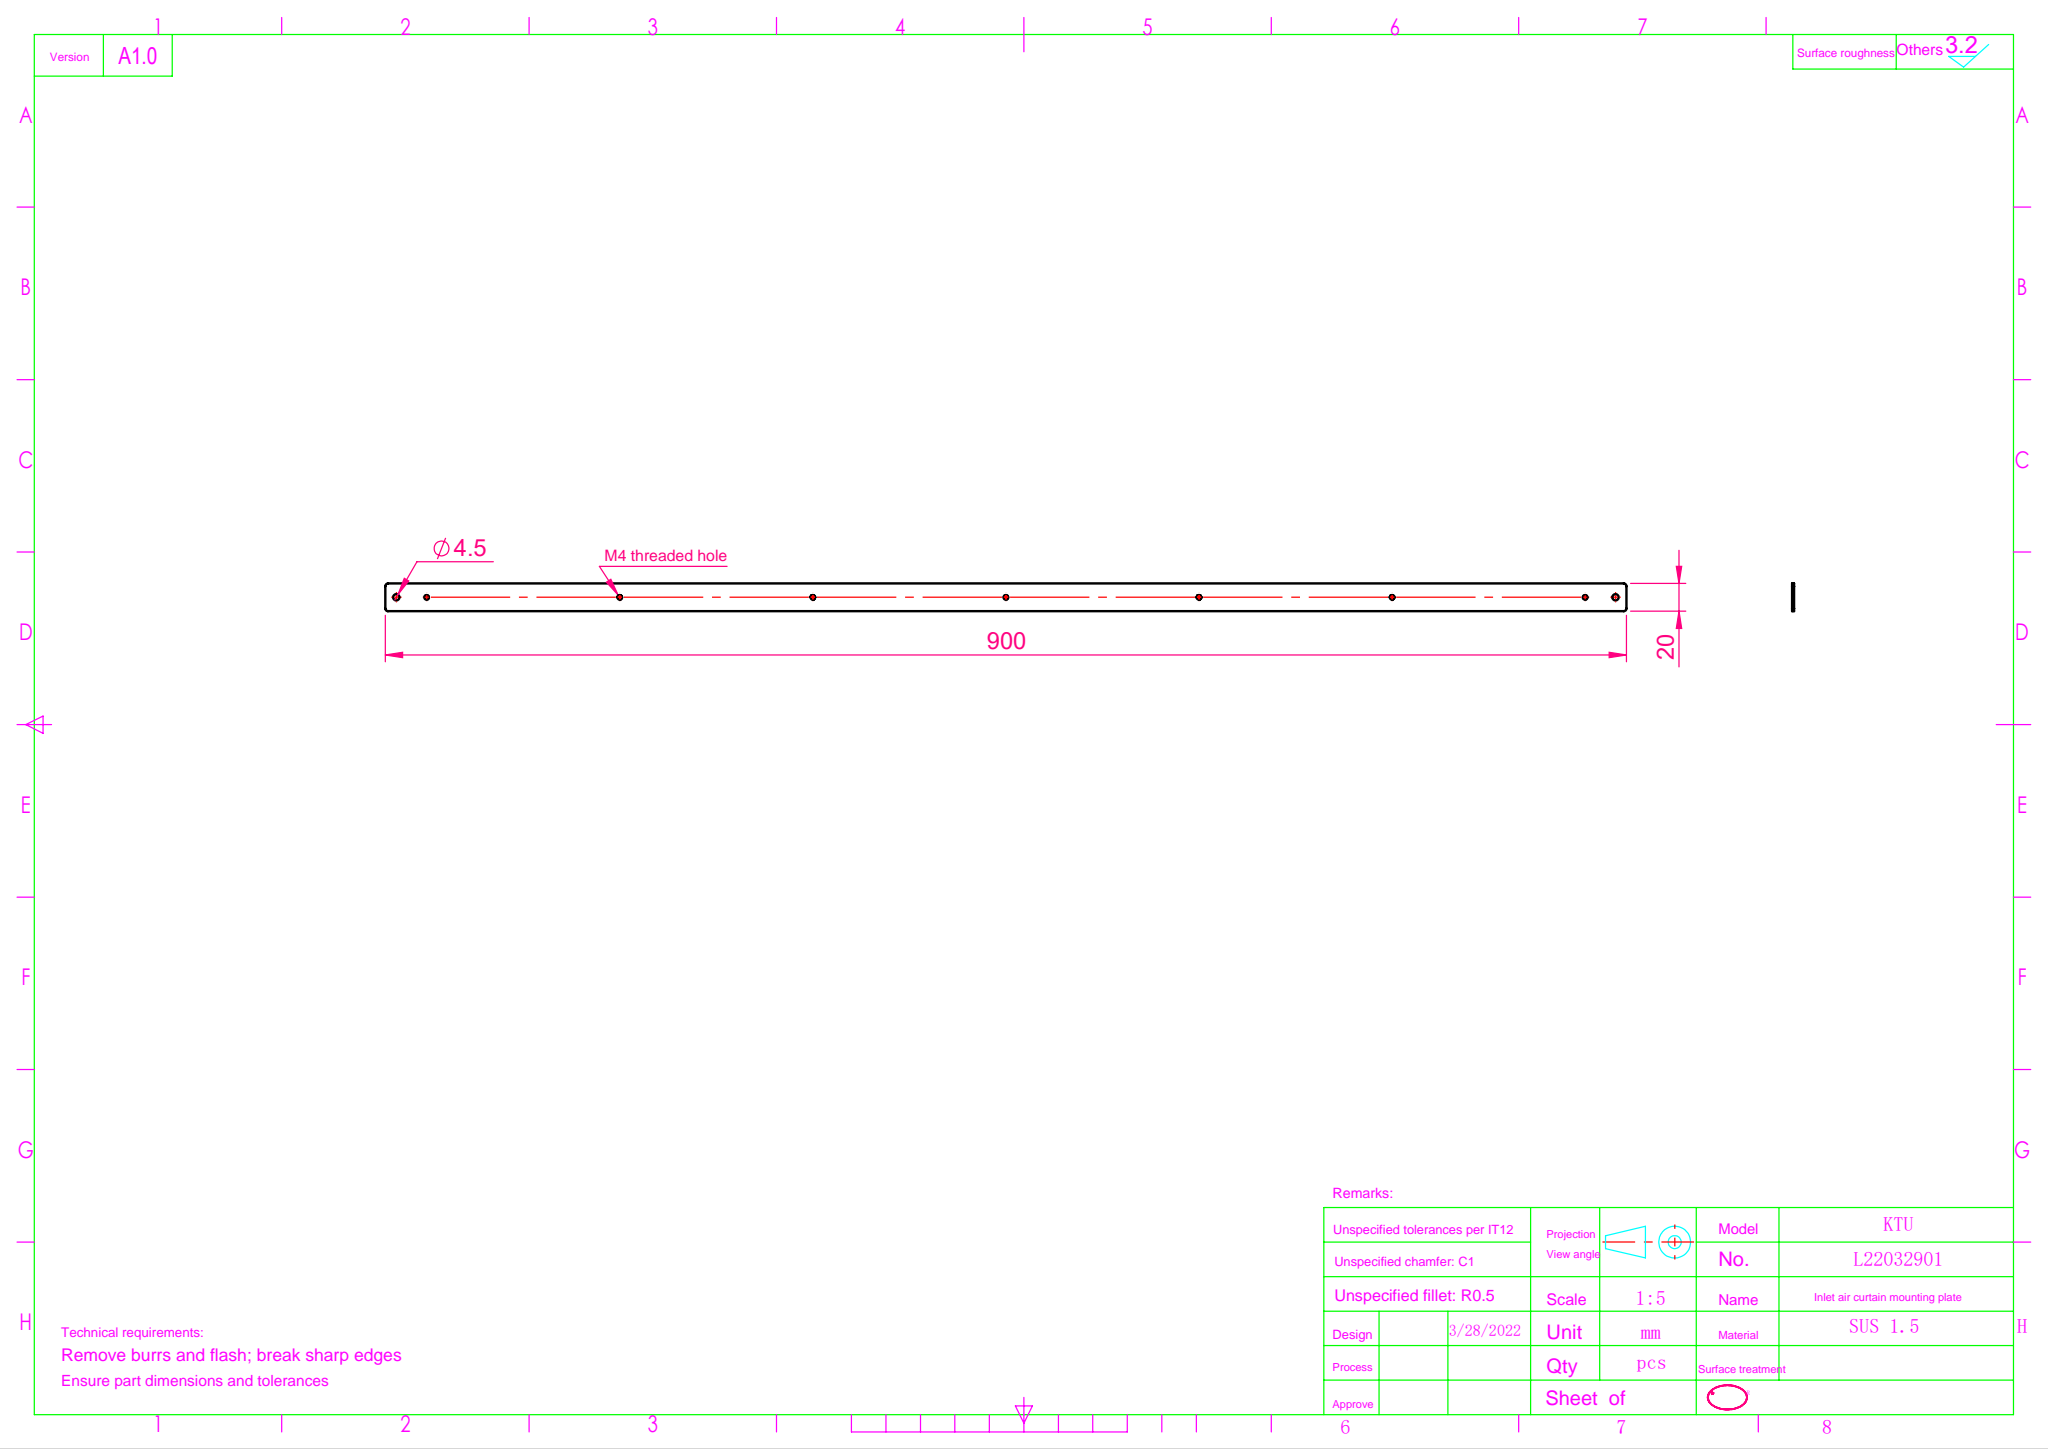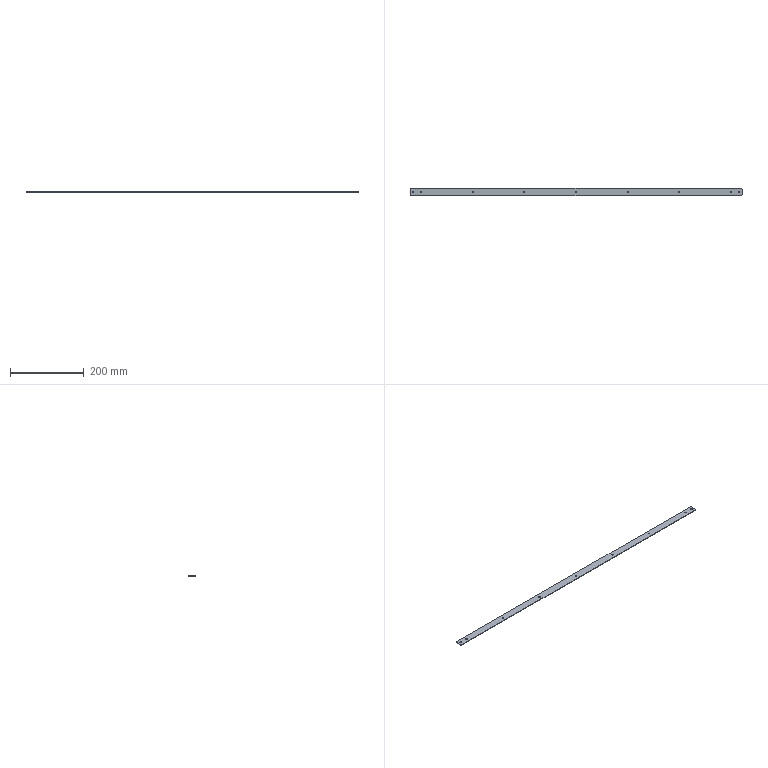Part | SolidWorks | features Fillet 1, FlatPattern 1, HoleWzd 1, ICE 1, LPattern 1, SMBaseFlange 1, SheetMetal 1 | 1 solid | 28 faces | box 900 x 20 x 1.5 mm | volume 26857 mm3 | cylinder 22 | plane 6 | commonest cylinder face diameters 3.3 x14 4 x4 4.5 x4
STEP:
#1=CARTESIAN_POINT('',(444.25,0.,-1.5));
#2=VERTEX_POINT('',#1);
#3=CARTESIAN_POINT('',(439.75,0.,-1.5));
#4=VERTEX_POINT('',#3);
#5=CARTESIAN_POINT('',(442.,0.,-1.5));
#6=DIRECTION('',(0.,0.,-1.));
#7=DIRECTION('',(1.,0.,0.));
#8=AXIS2_PLACEMENT_3D('',#5,#6,#7);
#9=CIRCLE('',#8,2.25);
#10=EDGE_CURVE('',#2,#4,#9,.T.);
#11=ORIENTED_EDGE('',*,*,#10,.T.);
#12=CARTESIAN_POINT('',(439.75,0.,0.));
#13=VERTEX_POINT('',#12);
#14=CARTESIAN_POINT('',(439.75,0.,-1.501));
#15=DIRECTION('',(0.,0.,1.));
#16=VECTOR('',#15,1000.);
#17=LINE('',#14,#16);
#18=EDGE_CURVE('',#4,#13,#17,.T.);
#19=ORIENTED_EDGE('',*,*,#18,.T.);
#20=CARTESIAN_POINT('',(444.25,0.,0.));
#21=VERTEX_POINT('',#20);
#22=CARTESIAN_POINT('',(442.,0.,0.));
#23=DIRECTION('',(0.,0.,1.));
#24=DIRECTION('',(-1.,0.,0.));
#25=AXIS2_PLACEMENT_3D('',#22,#23,#24);
#26=CIRCLE('',#25,2.25);
#27=EDGE_CURVE('',#13,#21,#26,.T.);
#28=ORIENTED_EDGE('',*,*,#27,.T.);
#29=CARTESIAN_POINT('',(444.25,0.,-1.501));
#30=DIRECTION('',(0.,0.,1.));
#31=VECTOR('',#30,1000.);
#32=LINE('',#29,#31);
#33=EDGE_CURVE('',#2,#21,#32,.T.);
#34=ORIENTED_EDGE('',*,*,#33,.F.);
#35=EDGE_LOOP('',(#11,#19,#28,#34));
#36=FACE_OUTER_BOUND('',#35,.T.);
#37=CARTESIAN_POINT('',(442.,0.,-1.501));
#38=DIRECTION('',(0.,0.,1.));
#39=DIRECTION('',(1.,0.,0.));
#40=AXIS2_PLACEMENT_3D('',#37,#38,#39);
#41=CYLINDRICAL_SURFACE('',#40,2.25);
#42=ADVANCED_FACE('',(#36),#41,.F.);
#43=CARTESIAN_POINT('',(-439.75,0.,-1.5));
#44=VERTEX_POINT('',#43);
#45=CARTESIAN_POINT('',(-444.25,0.,-1.5));
#46=VERTEX_POINT('',#45);
#47=CARTESIAN_POINT('',(-442.,0.,-1.5));
#48=DIRECTION('',(0.,0.,-1.));
#49=DIRECTION('',(1.,0.,0.));
#50=AXIS2_PLACEMENT_3D('',#47,#48,#49);
#51=CIRCLE('',#50,2.25);
#52=EDGE_CURVE('',#44,#46,#51,.T.);
#53=ORIENTED_EDGE('',*,*,#52,.T.);
#54=CARTESIAN_POINT('',(-444.25,0.,0.));
#55=VERTEX_POINT('',#54);
#56=CARTESIAN_POINT('',(-444.25,0.,-1.501));
#57=DIRECTION('',(0.,0.,1.));
#58=VECTOR('',#57,1000.);
#59=LINE('',#56,#58);
#60=EDGE_CURVE('',#46,#55,#59,.T.);
#61=ORIENTED_EDGE('',*,*,#60,.T.);
#62=CARTESIAN_POINT('',(-439.75,0.,0.));
#63=VERTEX_POINT('',#62);
#64=CARTESIAN_POINT('',(-442.,0.,0.));
#65=DIRECTION('',(0.,0.,1.));
#66=DIRECTION('',(1.,0.,0.));
#67=AXIS2_PLACEMENT_3D('',#64,#65,#66);
#68=CIRCLE('',#67,2.25);
#69=EDGE_CURVE('',#55,#63,#68,.T.);
#70=ORIENTED_EDGE('',*,*,#69,.T.);
#71=CARTESIAN_POINT('',(-439.75,0.,-1.501));
#72=DIRECTION('',(0.,0.,1.));
#73=VECTOR('',#72,1000.);
#74=LINE('',#71,#73);
#75=EDGE_CURVE('',#44,#63,#74,.T.);
#76=ORIENTED_EDGE('',*,*,#75,.F.);
#77=EDGE_LOOP('',(#53,#61,#70,#76));
#78=FACE_OUTER_BOUND('',#77,.T.);
#79=CARTESIAN_POINT('',(-442.,0.,-1.501));
#80=DIRECTION('',(0.,0.,1.));
#81=DIRECTION('',(1.,0.,0.));
#82=AXIS2_PLACEMENT_3D('',#79,#80,#81);
#83=CYLINDRICAL_SURFACE('',#82,2.25);
#84=ADVANCED_FACE('',(#78),#83,.F.);
#85=CARTESIAN_POINT('',(418.35,0.,-1.5));
#86=VERTEX_POINT('',#85);
#87=CARTESIAN_POINT('',(421.65,0.,-1.5));
#88=VERTEX_POINT('',#87);
#89=CARTESIAN_POINT('',(420.,0.,-1.5));
#90=DIRECTION('',(0.,0.,1.));
#91=DIRECTION('',(1.,0.,0.));
#92=AXIS2_PLACEMENT_3D('',#89,#90,#91);
#93=CIRCLE('',#92,1.65);
#94=EDGE_CURVE('',#86,#88,#93,.T.);
#95=ORIENTED_EDGE('',*,*,#94,.F.);
#96=CARTESIAN_POINT('',(418.35,0.,0.));
#97=VERTEX_POINT('',#96);
#98=CARTESIAN_POINT('',(418.35,0.,0.));
#99=DIRECTION('',(0.,0.,1.));
#100=VECTOR('',#99,1000.);
#101=LINE('',#98,#100);
#102=EDGE_CURVE('',#86,#97,#101,.T.);
#103=ORIENTED_EDGE('',*,*,#102,.T.);
#104=CARTESIAN_POINT('',(421.65,0.,0.));
#105=VERTEX_POINT('',#104);
#106=CARTESIAN_POINT('',(420.,0.,0.));
#107=DIRECTION('',(0.,0.,1.));
#108=DIRECTION('',(1.,0.,0.));
#109=AXIS2_PLACEMENT_3D('',#106,#107,#108);
#110=CIRCLE('',#109,1.65);
#111=EDGE_CURVE('',#97,#105,#110,.T.);
#112=ORIENTED_EDGE('',*,*,#111,.T.);
#113=CARTESIAN_POINT('',(421.65,0.,0.));
#114=DIRECTION('',(0.,0.,1.));
#115=VECTOR('',#114,1000.);
#116=LINE('',#113,#115);
#117=EDGE_CURVE('',#88,#105,#116,.T.);
#118=ORIENTED_EDGE('',*,*,#117,.F.);
#119=EDGE_LOOP('',(#95,#103,#112,#118));
#120=FACE_OUTER_BOUND('',#119,.T.);
#121=CARTESIAN_POINT('',(420.,0.,0.));
#122=DIRECTION('',(0.,0.,1.));
#123=DIRECTION('',(1.,0.,0.));
#124=AXIS2_PLACEMENT_3D('',#121,#122,#123);
#125=CYLINDRICAL_SURFACE('',#124,1.65);
#126=ADVANCED_FACE('',(#120),#125,.F.);
#127=CARTESIAN_POINT('',(278.35,0.,-1.5));
#128=VERTEX_POINT('',#127);
#129=CARTESIAN_POINT('',(281.65,0.,-1.5));
#130=VERTEX_POINT('',#129);
#131=CARTESIAN_POINT('',(280.,0.,-1.5));
#132=DIRECTION('',(0.,0.,1.));
#133=DIRECTION('',(1.,0.,0.));
#134=AXIS2_PLACEMENT_3D('',#131,#132,#133);
#135=CIRCLE('',#134,1.65);
#136=EDGE_CURVE('',#128,#130,#135,.T.);
#137=ORIENTED_EDGE('',*,*,#136,.F.);
#138=CARTESIAN_POINT('',(278.35,0.,0.));
#139=VERTEX_POINT('',#138);
#140=CARTESIAN_POINT('',(278.35,0.,0.));
#141=DIRECTION('',(0.,0.,1.));
#142=VECTOR('',#141,1000.);
#143=LINE('',#140,#142);
#144=EDGE_CURVE('',#128,#139,#143,.T.);
#145=ORIENTED_EDGE('',*,*,#144,.T.);
#146=CARTESIAN_POINT('',(281.65,0.,0.));
#147=VERTEX_POINT('',#146);
#148=CARTESIAN_POINT('',(280.,0.,0.));
#149=DIRECTION('',(0.,0.,1.));
#150=DIRECTION('',(1.,0.,0.));
#151=AXIS2_PLACEMENT_3D('',#148,#149,#150);
#152=CIRCLE('',#151,1.65);
#153=EDGE_CURVE('',#139,#147,#152,.T.);
#154=ORIENTED_EDGE('',*,*,#153,.T.);
#155=CARTESIAN_POINT('',(281.65,0.,0.));
#156=DIRECTION('',(0.,0.,1.));
#157=VECTOR('',#156,1000.);
#158=LINE('',#155,#157);
#159=EDGE_CURVE('',#130,#147,#158,.T.);
#160=ORIENTED_EDGE('',*,*,#159,.F.);
#161=EDGE_LOOP('',(#137,#145,#154,#160));
#162=FACE_OUTER_BOUND('',#161,.T.);
#163=CARTESIAN_POINT('',(280.,0.,0.));
#164=DIRECTION('',(0.,0.,1.));
#165=DIRECTION('',(1.,0.,0.));
#166=AXIS2_PLACEMENT_3D('',#163,#164,#165);
#167=CYLINDRICAL_SURFACE('',#166,1.65);
#168=ADVANCED_FACE('',(#162),#167,.F.);
#169=CARTESIAN_POINT('',(138.35,0.,-1.5));
#170=VERTEX_POINT('',#169);
#171=CARTESIAN_POINT('',(141.65,0.,-1.5));
#172=VERTEX_POINT('',#171);
#173=CARTESIAN_POINT('',(140.,0.,-1.5));
#174=DIRECTION('',(0.,0.,1.));
#175=DIRECTION('',(1.,0.,0.));
#176=AXIS2_PLACEMENT_3D('',#173,#174,#175);
#177=CIRCLE('',#176,1.65);
#178=EDGE_CURVE('',#170,#172,#177,.T.);
#179=ORIENTED_EDGE('',*,*,#178,.F.);
#180=CARTESIAN_POINT('',(138.35,0.,0.));
#181=VERTEX_POINT('',#180);
#182=CARTESIAN_POINT('',(138.35,0.,0.));
#183=DIRECTION('',(0.,0.,1.));
#184=VECTOR('',#183,1000.);
#185=LINE('',#182,#184);
#186=EDGE_CURVE('',#170,#181,#185,.T.);
#187=ORIENTED_EDGE('',*,*,#186,.T.);
#188=CARTESIAN_POINT('',(141.65,0.,0.));
#189=VERTEX_POINT('',#188);
#190=CARTESIAN_POINT('',(140.,0.,0.));
#191=DIRECTION('',(0.,0.,1.));
#192=DIRECTION('',(1.,0.,0.));
#193=AXIS2_PLACEMENT_3D('',#190,#191,#192);
#194=CIRCLE('',#193,1.65);
#195=EDGE_CURVE('',#181,#189,#194,.T.);
#196=ORIENTED_EDGE('',*,*,#195,.T.);
#197=CARTESIAN_POINT('',(141.65,0.,0.));
#198=DIRECTION('',(0.,0.,1.));
#199=VECTOR('',#198,1000.);
#200=LINE('',#197,#199);
#201=EDGE_CURVE('',#172,#189,#200,.T.);
#202=ORIENTED_EDGE('',*,*,#201,.F.);
#203=EDGE_LOOP('',(#179,#187,#196,#202));
#204=FACE_OUTER_BOUND('',#203,.T.);
#205=CARTESIAN_POINT('',(140.,0.,0.));
#206=DIRECTION('',(0.,0.,1.));
#207=DIRECTION('',(1.,0.,0.));
#208=AXIS2_PLACEMENT_3D('',#205,#206,#207);
#209=CYLINDRICAL_SURFACE('',#208,1.65);
#210=ADVANCED_FACE('',(#204),#209,.F.);
#211=CARTESIAN_POINT('',(-421.65,0.,-1.5));
#212=VERTEX_POINT('',#211);
#213=CARTESIAN_POINT('',(-418.35,0.,-1.5));
#214=VERTEX_POINT('',#213);
#215=CARTESIAN_POINT('',(-420.,0.,-1.5));
#216=DIRECTION('',(0.,0.,1.));
#217=DIRECTION('',(1.,0.,0.));
#218=AXIS2_PLACEMENT_3D('',#215,#216,#217);
#219=CIRCLE('',#218,1.65);
#220=EDGE_CURVE('',#212,#214,#219,.T.);
#221=ORIENTED_EDGE('',*,*,#220,.F.);
#222=CARTESIAN_POINT('',(-421.65,0.,0.));
#223=VERTEX_POINT('',#222);
#224=CARTESIAN_POINT('',(-421.65,0.,0.));
#225=DIRECTION('',(0.,0.,1.));
#226=VECTOR('',#225,1000.);
#227=LINE('',#224,#226);
#228=EDGE_CURVE('',#212,#223,#227,.T.);
#229=ORIENTED_EDGE('',*,*,#228,.T.);
#230=CARTESIAN_POINT('',(-418.35,0.,0.));
#231=VERTEX_POINT('',#230);
#232=CARTESIAN_POINT('',(-420.,0.,0.));
#233=DIRECTION('',(0.,0.,1.));
#234=DIRECTION('',(1.,0.,0.));
#235=AXIS2_PLACEMENT_3D('',#232,#233,#234);
#236=CIRCLE('',#235,1.65);
#237=EDGE_CURVE('',#223,#231,#236,.T.);
#238=ORIENTED_EDGE('',*,*,#237,.T.);
#239=CARTESIAN_POINT('',(-418.35,0.,0.));
#240=DIRECTION('',(0.,0.,1.));
#241=VECTOR('',#240,1000.);
#242=LINE('',#239,#241);
#243=EDGE_CURVE('',#214,#231,#242,.T.);
#244=ORIENTED_EDGE('',*,*,#243,.F.);
#245=EDGE_LOOP('',(#221,#229,#238,#244));
#246=FACE_OUTER_BOUND('',#245,.T.);
#247=CARTESIAN_POINT('',(-420.,0.,0.));
#248=DIRECTION('',(0.,0.,1.));
#249=DIRECTION('',(1.,0.,0.));
#250=AXIS2_PLACEMENT_3D('',#247,#248,#249);
#251=CYLINDRICAL_SURFACE('',#250,1.65);
#252=ADVANCED_FACE('',(#246),#251,.F.);
#253=CARTESIAN_POINT('',(-281.65,0.,-1.5));
#254=VERTEX_POINT('',#253);
#255=CARTESIAN_POINT('',(-278.35,0.,-1.5));
#256=VERTEX_POINT('',#255);
#257=CARTESIAN_POINT('',(-280.,0.,-1.5));
#258=DIRECTION('',(0.,0.,1.));
#259=DIRECTION('',(1.,0.,0.));
#260=AXIS2_PLACEMENT_3D('',#257,#258,#259);
#261=CIRCLE('',#260,1.65);
#262=EDGE_CURVE('',#254,#256,#261,.T.);
#263=ORIENTED_EDGE('',*,*,#262,.F.);
#264=CARTESIAN_POINT('',(-281.65,0.,0.));
#265=VERTEX_POINT('',#264);
#266=CARTESIAN_POINT('',(-281.65,0.,0.));
#267=DIRECTION('',(0.,0.,1.));
#268=VECTOR('',#267,1000.);
#269=LINE('',#266,#268);
#270=EDGE_CURVE('',#254,#265,#269,.T.);
#271=ORIENTED_EDGE('',*,*,#270,.T.);
#272=CARTESIAN_POINT('',(-278.35,0.,0.));
#273=VERTEX_POINT('',#272);
#274=CARTESIAN_POINT('',(-280.,0.,0.));
#275=DIRECTION('',(0.,0.,1.));
#276=DIRECTION('',(1.,0.,0.));
#277=AXIS2_PLACEMENT_3D('',#274,#275,#276);
#278=CIRCLE('',#277,1.65);
#279=EDGE_CURVE('',#265,#273,#278,.T.);
#280=ORIENTED_EDGE('',*,*,#279,.T.);
#281=CARTESIAN_POINT('',(-278.35,0.,0.));
#282=DIRECTION('',(0.,0.,1.));
#283=VECTOR('',#282,1000.);
#284=LINE('',#281,#283);
#285=EDGE_CURVE('',#256,#273,#284,.T.);
#286=ORIENTED_EDGE('',*,*,#285,.F.);
#287=EDGE_LOOP('',(#263,#271,#280,#286));
#288=FACE_OUTER_BOUND('',#287,.T.);
#289=CARTESIAN_POINT('',(-280.,0.,0.));
#290=DIRECTION('',(0.,0.,1.));
#291=DIRECTION('',(1.,0.,0.));
#292=AXIS2_PLACEMENT_3D('',#289,#290,#291);
#293=CYLINDRICAL_SURFACE('',#292,1.65);
#294=ADVANCED_FACE('',(#288),#293,.F.);
#295=CARTESIAN_POINT('',(-141.65,0.,-1.5));
#296=VERTEX_POINT('',#295);
#297=CARTESIAN_POINT('',(-138.35,0.,-1.5));
#298=VERTEX_POINT('',#297);
#299=CARTESIAN_POINT('',(-140.,0.,-1.5));
#300=DIRECTION('',(0.,0.,1.));
#301=DIRECTION('',(1.,0.,0.));
#302=AXIS2_PLACEMENT_3D('',#299,#300,#301);
#303=CIRCLE('',#302,1.65);
#304=EDGE_CURVE('',#296,#298,#303,.T.);
#305=ORIENTED_EDGE('',*,*,#304,.F.);
#306=CARTESIAN_POINT('',(-141.65,0.,0.));
#307=VERTEX_POINT('',#306);
#308=CARTESIAN_POINT('',(-141.65,0.,0.));
#309=DIRECTION('',(0.,0.,1.));
#310=VECTOR('',#309,1000.);
#311=LINE('',#308,#310);
#312=EDGE_CURVE('',#296,#307,#311,.T.);
#313=ORIENTED_EDGE('',*,*,#312,.T.);
#314=CARTESIAN_POINT('',(-138.35,0.,0.));
#315=VERTEX_POINT('',#314);
#316=CARTESIAN_POINT('',(-140.,0.,0.));
#317=DIRECTION('',(0.,0.,1.));
#318=DIRECTION('',(1.,0.,0.));
#319=AXIS2_PLACEMENT_3D('',#316,#317,#318);
#320=CIRCLE('',#319,1.65);
#321=EDGE_CURVE('',#307,#315,#320,.T.);
#322=ORIENTED_EDGE('',*,*,#321,.T.);
#323=CARTESIAN_POINT('',(-138.35,0.,0.));
#324=DIRECTION('',(0.,0.,1.));
#325=VECTOR('',#324,1000.);
#326=LINE('',#323,#325);
#327=EDGE_CURVE('',#298,#315,#326,.T.);
#328=ORIENTED_EDGE('',*,*,#327,.F.);
#329=EDGE_LOOP('',(#305,#313,#322,#328));
#330=FACE_OUTER_BOUND('',#329,.T.);
#331=CARTESIAN_POINT('',(-140.,0.,0.));
#332=DIRECTION('',(0.,0.,1.));
#333=DIRECTION('',(1.,0.,0.));
#334=AXIS2_PLACEMENT_3D('',#331,#332,#333);
#335=CYLINDRICAL_SURFACE('',#334,1.65);
#336=ADVANCED_FACE('',(#330),#335,.F.);
#337=CARTESIAN_POINT('',(-1.65,0.,-1.5));
#338=VERTEX_POINT('',#337);
#339=CARTESIAN_POINT('',(1.65,0.,-1.5));
#340=VERTEX_POINT('',#339);
#341=CARTESIAN_POINT('',(0.,0.,-1.5));
#342=DIRECTION('',(0.,0.,1.));
#343=DIRECTION('',(1.,0.,0.));
#344=AXIS2_PLACEMENT_3D('',#341,#342,#343);
#345=CIRCLE('',#344,1.65);
#346=EDGE_CURVE('',#338,#340,#345,.T.);
#347=ORIENTED_EDGE('',*,*,#346,.F.);
#348=CARTESIAN_POINT('',(-1.65,0.,0.));
#349=VERTEX_POINT('',#348);
#350=CARTESIAN_POINT('',(-1.65,0.,0.));
#351=DIRECTION('',(0.,0.,1.));
#352=VECTOR('',#351,1000.);
#353=LINE('',#350,#352);
#354=EDGE_CURVE('',#338,#349,#353,.T.);
#355=ORIENTED_EDGE('',*,*,#354,.T.);
#356=CARTESIAN_POINT('',(1.65,0.,0.));
#357=VERTEX_POINT('',#356);
#358=CARTESIAN_POINT('',(0.,0.,0.));
#359=DIRECTION('',(0.,0.,1.));
#360=DIRECTION('',(1.,0.,0.));
#361=AXIS2_PLACEMENT_3D('',#358,#359,#360);
#362=CIRCLE('',#361,1.65);
#363=EDGE_CURVE('',#349,#357,#362,.T.);
#364=ORIENTED_EDGE('',*,*,#363,.T.);
#365=CARTESIAN_POINT('',(1.65,0.,0.));
#366=DIRECTION('',(0.,0.,1.));
#367=VECTOR('',#366,1000.);
#368=LINE('',#365,#367);
#369=EDGE_CURVE('',#340,#357,#368,.T.);
#370=ORIENTED_EDGE('',*,*,#369,.F.);
#371=EDGE_LOOP('',(#347,#355,#364,#370));
#372=FACE_OUTER_BOUND('',#371,.T.);
#373=CARTESIAN_POINT('',(0.,0.,0.));
#374=DIRECTION('',(0.,0.,1.));
#375=DIRECTION('',(1.,0.,0.));
#376=AXIS2_PLACEMENT_3D('',#373,#374,#375);
#377=CYLINDRICAL_SURFACE('',#376,1.65);
#378=ADVANCED_FACE('',(#372),#377,.F.);
#379=CARTESIAN_POINT('',(450.,-8.,0.));
#380=VERTEX_POINT('',#379);
#381=CARTESIAN_POINT('',(450.,8.,0.));
#382=VERTEX_POINT('',#381);
#383=CARTESIAN_POINT('',(450.,10.,0.));
#384=DIRECTION('',(0.,1.,0.));
#385=VECTOR('',#384,1000.);
#386=LINE('',#383,#385);
#387=EDGE_CURVE('',#380,#382,#386,.T.);
#388=ORIENTED_EDGE('',*,*,#387,.F.);
#389=CARTESIAN_POINT('',(450.,-8.,-1.5));
#390=VERTEX_POINT('',#389);
#391=CARTESIAN_POINT('',(450.,-8.,-1.5));
#392=DIRECTION('',(0.,0.,-1.));
#393=VECTOR('',#392,1000.);
#394=LINE('',#391,#393);
#395=EDGE_CURVE('',#380,#390,#394,.T.);
#396=ORIENTED_EDGE('',*,*,#395,.T.);
#397=CARTESIAN_POINT('',(450.,8.,-1.5));
#398=VERTEX_POINT('',#397);
#399=CARTESIAN_POINT('',(450.,10.,-1.5));
#400=DIRECTION('',(0.,1.,0.));
#401=VECTOR('',#400,1000.);
#402=LINE('',#399,#401);
#403=EDGE_CURVE('',#390,#398,#402,.T.);
#404=ORIENTED_EDGE('',*,*,#403,.T.);
#405=CARTESIAN_POINT('',(450.,8.,-1.5));
#406=DIRECTION('',(0.,0.,1.));
#407=VECTOR('',#406,1000.);
#408=LINE('',#405,#407);
#409=EDGE_CURVE('',#398,#382,#408,.T.);
#410=ORIENTED_EDGE('',*,*,#409,.T.);
#411=EDGE_LOOP('',(#388,#396,#404,#410));
#412=FACE_OUTER_BOUND('',#411,.T.);
#413=CARTESIAN_POINT('',(450.,10.,-1.5));
#414=DIRECTION('',(1.,0.,0.));
#415=DIRECTION('',(0.,1.,0.));
#416=AXIS2_PLACEMENT_3D('',#413,#414,#415);
#417=PLANE('',#416);
#418=ADVANCED_FACE('',(#412),#417,.T.);
#419=CARTESIAN_POINT('',(-448.,-10.,0.));
#420=VERTEX_POINT('',#419);
#421=CARTESIAN_POINT('',(448.,-10.,0.));
#422=VERTEX_POINT('',#421);
#423=CARTESIAN_POINT('',(-450.,-10.,0.));
#424=DIRECTION('',(1.,0.,0.));
#425=VECTOR('',#424,1000.);
#426=LINE('',#423,#425);
#427=EDGE_CURVE('',#420,#422,#426,.T.);
#428=ORIENTED_EDGE('',*,*,#427,.F.);
#429=CARTESIAN_POINT('',(-448.,-10.,-1.5));
#430=VERTEX_POINT('',#429);
#431=CARTESIAN_POINT('',(-448.,-10.,-1.5));
#432=DIRECTION('',(0.,0.,-1.));
#433=VECTOR('',#432,1000.);
#434=LINE('',#431,#433);
#435=EDGE_CURVE('',#420,#430,#434,.T.);
#436=ORIENTED_EDGE('',*,*,#435,.T.);
#437=CARTESIAN_POINT('',(448.,-10.,-1.5));
#438=VERTEX_POINT('',#437);
#439=CARTESIAN_POINT('',(-450.,-10.,-1.5));
#440=DIRECTION('',(1.,0.,0.));
#441=VECTOR('',#440,1000.);
#442=LINE('',#439,#441);
#443=EDGE_CURVE('',#430,#438,#442,.T.);
#444=ORIENTED_EDGE('',*,*,#443,.T.);
#445=CARTESIAN_POINT('',(448.,-10.,-1.5));
#446=DIRECTION('',(0.,0.,1.));
#447=VECTOR('',#446,1000.);
#448=LINE('',#445,#447);
#449=EDGE_CURVE('',#438,#422,#448,.T.);
#450=ORIENTED_EDGE('',*,*,#449,.T.);
#451=EDGE_LOOP('',(#428,#436,#444,#450));
#452=FACE_OUTER_BOUND('',#451,.T.);
#453=CARTESIAN_POINT('',(-450.,-10.,-1.5));
#454=DIRECTION('',(0.,-1.,0.));
#455=DIRECTION('',(0.,0.,-1.));
#456=AXIS2_PLACEMENT_3D('',#453,#454,#455);
#457=PLANE('',#456);
#458=ADVANCED_FACE('',(#452),#457,.T.);
#459=CARTESIAN_POINT('',(-450.,8.,-1.5));
#460=VERTEX_POINT('',#459);
#461=CARTESIAN_POINT('',(-450.,-8.,-1.5));
#462=VERTEX_POINT('',#461);
#463=CARTESIAN_POINT('',(-450.,10.,-1.5));
#464=DIRECTION('',(0.,-1.,0.));
#465=VECTOR('',#464,1000.);
#466=LINE('',#463,#465);
#467=EDGE_CURVE('',#460,#462,#466,.T.);
#468=ORIENTED_EDGE('',*,*,#467,.T.);
#469=CARTESIAN_POINT('',(-450.,-8.,0.));
#470=VERTEX_POINT('',#469);
#471=CARTESIAN_POINT('',(-450.,-8.,-1.5));
#472=DIRECTION('',(0.,0.,1.));
#473=VECTOR('',#472,1000.);
#474=LINE('',#471,#473);
#475=EDGE_CURVE('',#462,#470,#474,.T.);
#476=ORIENTED_EDGE('',*,*,#475,.T.);
#477=CARTESIAN_POINT('',(-450.,8.,0.));
#478=VERTEX_POINT('',#477);
#479=CARTESIAN_POINT('',(-450.,10.,0.));
#480=DIRECTION('',(0.,-1.,0.));
#481=VECTOR('',#480,1000.);
#482=LINE('',#479,#481);
#483=EDGE_CURVE('',#478,#470,#482,.T.);
#484=ORIENTED_EDGE('',*,*,#483,.F.);
#485=CARTESIAN_POINT('',(-450.,8.,-1.5));
#486=DIRECTION('',(0.,0.,-1.));
#487=VECTOR('',#486,1000.);
#488=LINE('',#485,#487);
#489=EDGE_CURVE('',#478,#460,#488,.T.);
#490=ORIENTED_EDGE('',*,*,#489,.T.);
#491=EDGE_LOOP('',(#468,#476,#484,#490));
#492=FACE_OUTER_BOUND('',#491,.T.);
#493=CARTESIAN_POINT('',(-450.,10.,-1.5));
#494=DIRECTION('',(-1.,0.,0.));
#495=DIRECTION('',(0.,0.,1.));
#496=AXIS2_PLACEMENT_3D('',#493,#494,#495);
#497=PLANE('',#496);
#498=ADVANCED_FACE('',(#492),#497,.T.);
#499=CARTESIAN_POINT('',(448.,10.,-1.5));
#500=VERTEX_POINT('',#499);
#501=CARTESIAN_POINT('',(-448.,10.,-1.5));
#502=VERTEX_POINT('',#501);
#503=CARTESIAN_POINT('',(-450.,10.,-1.5));
#504=DIRECTION('',(-1.,0.,0.));
#505=VECTOR('',#504,1000.);
#506=LINE('',#503,#505);
#507=EDGE_CURVE('',#500,#502,#506,.T.);
#508=ORIENTED_EDGE('',*,*,#507,.T.);
#509=CARTESIAN_POINT('',(-448.,10.,0.));
#510=VERTEX_POINT('',#509);
#511=CARTESIAN_POINT('',(-448.,10.,-1.5));
#512=DIRECTION('',(0.,0.,1.));
#513=VECTOR('',#512,1000.);
#514=LINE('',#511,#513);
#515=EDGE_CURVE('',#502,#510,#514,.T.);
#516=ORIENTED_EDGE('',*,*,#515,.T.);
#517=CARTESIAN_POINT('',(448.,10.,0.));
#518=VERTEX_POINT('',#517);
#519=CARTESIAN_POINT('',(-450.,10.,0.));
#520=DIRECTION('',(-1.,0.,0.));
#521=VECTOR('',#520,1000.);
#522=LINE('',#519,#521);
#523=EDGE_CURVE('',#518,#510,#522,.T.);
#524=ORIENTED_EDGE('',*,*,#523,.F.);
#525=CARTESIAN_POINT('',(448.,10.,-1.5));
#526=DIRECTION('',(0.,0.,-1.));
#527=VECTOR('',#526,1000.);
#528=LINE('',#525,#527);
#529=EDGE_CURVE('',#518,#500,#528,.T.);
#530=ORIENTED_EDGE('',*,*,#529,.T.);
#531=EDGE_LOOP('',(#508,#516,#524,#530));
#532=FACE_OUTER_BOUND('',#531,.T.);
#533=CARTESIAN_POINT('',(-450.,10.,-1.5));
#534=DIRECTION('',(0.,1.,0.));
#535=DIRECTION('',(0.,0.,1.));
#536=AXIS2_PLACEMENT_3D('',#533,#534,#535);
#537=PLANE('',#536);
#538=ADVANCED_FACE('',(#532),#537,.T.);
#539=ORIENTED_EDGE('',*,*,#10,.F.);
#540=CARTESIAN_POINT('',(442.,0.,-1.5));
#541=DIRECTION('',(0.,0.,-1.));
#542=DIRECTION('',(1.,0.,0.));
#543=AXIS2_PLACEMENT_3D('',#540,#541,#542);
#544=CIRCLE('',#543,2.25);
#545=EDGE_CURVE('',#4,#2,#544,.T.);
#546=ORIENTED_EDGE('',*,*,#545,.F.);
#547=EDGE_LOOP('',(#539,#546));
#548=FACE_BOUND('',#547,.T.);
#549=ORIENTED_EDGE('',*,*,#52,.F.);
#550=CARTESIAN_POINT('',(-442.,0.,-1.5));
#551=DIRECTION('',(0.,0.,-1.));
#552=DIRECTION('',(1.,0.,0.));
#553=AXIS2_PLACEMENT_3D('',#550,#551,#552);
#554=CIRCLE('',#553,2.25);
#555=EDGE_CURVE('',#46,#44,#554,.T.);
#556=ORIENTED_EDGE('',*,*,#555,.F.);
#557=EDGE_LOOP('',(#549,#556));
#558=FACE_BOUND('',#557,.T.);
#559=CARTESIAN_POINT('',(420.,0.,-1.5));
#560=DIRECTION('',(0.,0.,1.));
#561=DIRECTION('',(1.,0.,0.));
#562=AXIS2_PLACEMENT_3D('',#559,#560,#561);
#563=CIRCLE('',#562,1.65);
#564=EDGE_CURVE('',#88,#86,#563,.T.);
#565=ORIENTED_EDGE('',*,*,#564,.T.);
#566=ORIENTED_EDGE('',*,*,#94,.T.);
#567=EDGE_LOOP('',(#565,#566));
#568=FACE_BOUND('',#567,.T.);
#569=CARTESIAN_POINT('',(280.,0.,-1.5));
#570=DIRECTION('',(0.,0.,1.));
#571=DIRECTION('',(1.,0.,0.));
#572=AXIS2_PLACEMENT_3D('',#569,#570,#571);
#573=CIRCLE('',#572,1.65);
#574=EDGE_CURVE('',#130,#128,#573,.T.);
#575=ORIENTED_EDGE('',*,*,#574,.T.);
#576=ORIENTED_EDGE('',*,*,#136,.T.);
#577=EDGE_LOOP('',(#575,#576));
#578=FACE_BOUND('',#577,.T.);
#579=CARTESIAN_POINT('',(140.,0.,-1.5));
#580=DIRECTION('',(0.,0.,1.));
#581=DIRECTION('',(1.,0.,0.));
#582=AXIS2_PLACEMENT_3D('',#579,#580,#581);
#583=CIRCLE('',#582,1.65);
#584=EDGE_CURVE('',#172,#170,#583,.T.);
#585=ORIENTED_EDGE('',*,*,#584,.T.);
#586=ORIENTED_EDGE('',*,*,#178,.T.);
#587=EDGE_LOOP('',(#585,#586));
#588=FACE_BOUND('',#587,.T.);
#589=CARTESIAN_POINT('',(-420.,0.,-1.5));
#590=DIRECTION('',(0.,0.,1.));
#591=DIRECTION('',(1.,0.,0.));
#592=AXIS2_PLACEMENT_3D('',#589,#590,#591);
#593=CIRCLE('',#592,1.65);
#594=EDGE_CURVE('',#214,#212,#593,.T.);
#595=ORIENTED_EDGE('',*,*,#594,.T.);
#596=ORIENTED_EDGE('',*,*,#220,.T.);
#597=EDGE_LOOP('',(#595,#596));
#598=FACE_BOUND('',#597,.T.);
#599=CARTESIAN_POINT('',(-280.,0.,-1.5));
#600=DIRECTION('',(0.,0.,1.));
#601=DIRECTION('',(1.,0.,0.));
#602=AXIS2_PLACEMENT_3D('',#599,#600,#601);
#603=CIRCLE('',#602,1.65);
#604=EDGE_CURVE('',#256,#254,#603,.T.);
#605=ORIENTED_EDGE('',*,*,#604,.T.);
#606=ORIENTED_EDGE('',*,*,#262,.T.);
#607=EDGE_LOOP('',(#605,#606));
#608=FACE_BOUND('',#607,.T.);
#609=CARTESIAN_POINT('',(-140.,0.,-1.5));
#610=DIRECTION('',(0.,0.,1.));
#611=DIRECTION('',(1.,0.,0.));
#612=AXIS2_PLACEMENT_3D('',#609,#610,#611);
#613=CIRCLE('',#612,1.65);
#614=EDGE_CURVE('',#298,#296,#613,.T.);
#615=ORIENTED_EDGE('',*,*,#614,.T.);
#616=ORIENTED_EDGE('',*,*,#304,.T.);
#617=EDGE_LOOP('',(#615,#616));
#618=FACE_BOUND('',#617,.T.);
#619=CARTESIAN_POINT('',(0.,0.,-1.5));
#620=DIRECTION('',(0.,0.,1.));
#621=DIRECTION('',(1.,0.,0.));
#622=AXIS2_PLACEMENT_3D('',#619,#620,#621);
#623=CIRCLE('',#622,1.65);
#624=EDGE_CURVE('',#340,#338,#623,.T.);
#625=ORIENTED_EDGE('',*,*,#624,.T.);
#626=ORIENTED_EDGE('',*,*,#346,.T.);
#627=EDGE_LOOP('',(#625,#626));
#628=FACE_BOUND('',#627,.T.);
#629=ORIENTED_EDGE('',*,*,#443,.F.);
#630=CARTESIAN_POINT('',(-448.,-8.,-1.5));
#631=DIRECTION('',(0.,0.,-1.));
#632=DIRECTION('',(1.,0.,0.));
#633=AXIS2_PLACEMENT_3D('',#630,#631,#632);
#634=CIRCLE('',#633,2.);
#635=EDGE_CURVE('',#430,#462,#634,.T.);
#636=ORIENTED_EDGE('',*,*,#635,.T.);
#637=ORIENTED_EDGE('',*,*,#467,.F.);
#638=CARTESIAN_POINT('',(-448.,8.,-1.5));
#639=DIRECTION('',(0.,0.,-1.));
#640=DIRECTION('',(1.,0.,0.));
#641=AXIS2_PLACEMENT_3D('',#638,#639,#640);
#642=CIRCLE('',#641,2.);
#643=EDGE_CURVE('',#460,#502,#642,.T.);
#644=ORIENTED_EDGE('',*,*,#643,.T.);
#645=ORIENTED_EDGE('',*,*,#507,.F.);
#646=CARTESIAN_POINT('',(448.,8.,-1.5));
#647=DIRECTION('',(0.,0.,-1.));
#648=DIRECTION('',(1.,0.,0.));
#649=AXIS2_PLACEMENT_3D('',#646,#647,#648);
#650=CIRCLE('',#649,2.);
#651=EDGE_CURVE('',#500,#398,#650,.T.);
#652=ORIENTED_EDGE('',*,*,#651,.T.);
#653=ORIENTED_EDGE('',*,*,#403,.F.);
#654=CARTESIAN_POINT('',(448.,-8.,-1.5));
#655=DIRECTION('',(0.,0.,-1.));
#656=DIRECTION('',(1.,0.,0.));
#657=AXIS2_PLACEMENT_3D('',#654,#655,#656);
#658=CIRCLE('',#657,2.);
#659=EDGE_CURVE('',#390,#438,#658,.T.);
#660=ORIENTED_EDGE('',*,*,#659,.T.);
#661=EDGE_LOOP('',(#629,#636,#637,#644,#645,#652,#653,#660));
#662=FACE_OUTER_BOUND('',#661,.T.);
#663=CARTESIAN_POINT('',(0.,0.,-1.5));
#664=DIRECTION('',(0.,0.,1.));
#665=DIRECTION('',(1.,0.,0.));
#666=AXIS2_PLACEMENT_3D('',#663,#664,#665);
#667=PLANE('',#666);
#668=ADVANCED_FACE('',(#548,#558,#568,#578,#588,#598,#608,#618,#628,#662),#667,.F.);
#669=CARTESIAN_POINT('',(442.,0.,0.));
#670=DIRECTION('',(0.,0.,1.));
#671=DIRECTION('',(-1.,0.,0.));
#672=AXIS2_PLACEMENT_3D('',#669,#670,#671);
#673=CIRCLE('',#672,2.25);
#674=EDGE_CURVE('',#21,#13,#673,.T.);
#675=ORIENTED_EDGE('',*,*,#674,.F.);
#676=ORIENTED_EDGE('',*,*,#27,.F.);
#677=EDGE_LOOP('',(#675,#676));
#678=FACE_BOUND('',#677,.T.);
#679=CARTESIAN_POINT('',(-442.,0.,0.));
#680=DIRECTION('',(0.,0.,1.));
#681=DIRECTION('',(1.,0.,0.));
#682=AXIS2_PLACEMENT_3D('',#679,#680,#681);
#683=CIRCLE('',#682,2.25);
#684=EDGE_CURVE('',#63,#55,#683,.T.);
#685=ORIENTED_EDGE('',*,*,#684,.F.);
#686=ORIENTED_EDGE('',*,*,#69,.F.);
#687=EDGE_LOOP('',(#685,#686));
#688=FACE_BOUND('',#687,.T.);
#689=CARTESIAN_POINT('',(420.,0.,0.));
#690=DIRECTION('',(0.,0.,1.));
#691=DIRECTION('',(1.,0.,0.));
#692=AXIS2_PLACEMENT_3D('',#689,#690,#691);
#693=CIRCLE('',#692,1.65);
#694=EDGE_CURVE('',#105,#97,#693,.T.);
#695=ORIENTED_EDGE('',*,*,#694,.F.);
#696=ORIENTED_EDGE('',*,*,#111,.F.);
#697=EDGE_LOOP('',(#695,#696));
#698=FACE_BOUND('',#697,.T.);
#699=CARTESIAN_POINT('',(280.,0.,0.));
#700=DIRECTION('',(0.,0.,1.));
#701=DIRECTION('',(1.,0.,0.));
#702=AXIS2_PLACEMENT_3D('',#699,#700,#701);
#703=CIRCLE('',#702,1.65);
#704=EDGE_CURVE('',#147,#139,#703,.T.);
#705=ORIENTED_EDGE('',*,*,#704,.F.);
#706=ORIENTED_EDGE('',*,*,#153,.F.);
#707=EDGE_LOOP('',(#705,#706));
#708=FACE_BOUND('',#707,.T.);
#709=CARTESIAN_POINT('',(140.,0.,0.));
#710=DIRECTION('',(0.,0.,1.));
#711=DIRECTION('',(1.,0.,0.));
#712=AXIS2_PLACEMENT_3D('',#709,#710,#711);
#713=CIRCLE('',#712,1.65);
#714=EDGE_CURVE('',#189,#181,#713,.T.);
#715=ORIENTED_EDGE('',*,*,#714,.F.);
#716=ORIENTED_EDGE('',*,*,#195,.F.);
#717=EDGE_LOOP('',(#715,#716));
#718=FACE_BOUND('',#717,.T.);
#719=CARTESIAN_POINT('',(-420.,0.,0.));
#720=DIRECTION('',(0.,0.,1.));
#721=DIRECTION('',(1.,0.,0.));
#722=AXIS2_PLACEMENT_3D('',#719,#720,#721);
#723=CIRCLE('',#722,1.65);
#724=EDGE_CURVE('',#231,#223,#723,.T.);
#725=ORIENTED_EDGE('',*,*,#724,.F.);
#726=ORIENTED_EDGE('',*,*,#237,.F.);
#727=EDGE_LOOP('',(#725,#726));
#728=FACE_BOUND('',#727,.T.);
#729=CARTESIAN_POINT('',(-280.,0.,0.));
#730=DIRECTION('',(0.,0.,1.));
#731=DIRECTION('',(1.,0.,0.));
#732=AXIS2_PLACEMENT_3D('',#729,#730,#731);
#733=CIRCLE('',#732,1.65);
#734=EDGE_CURVE('',#273,#265,#733,.T.);
#735=ORIENTED_EDGE('',*,*,#734,.F.);
#736=ORIENTED_EDGE('',*,*,#279,.F.);
#737=EDGE_LOOP('',(#735,#736));
#738=FACE_BOUND('',#737,.T.);
#739=CARTESIAN_POINT('',(-140.,0.,0.));
#740=DIRECTION('',(0.,0.,1.));
#741=DIRECTION('',(1.,0.,0.));
#742=AXIS2_PLACEMENT_3D('',#739,#740,#741);
#743=CIRCLE('',#742,1.65);
#744=EDGE_CURVE('',#315,#307,#743,.T.);
#745=ORIENTED_EDGE('',*,*,#744,.F.);
#746=ORIENTED_EDGE('',*,*,#321,.F.);
#747=EDGE_LOOP('',(#745,#746));
#748=FACE_BOUND('',#747,.T.);
#749=CARTESIAN_POINT('',(0.,0.,0.));
#750=DIRECTION('',(0.,0.,1.));
#751=DIRECTION('',(1.,0.,0.));
#752=AXIS2_PLACEMENT_3D('',#749,#750,#751);
#753=CIRCLE('',#752,1.65);
#754=EDGE_CURVE('',#357,#349,#753,.T.);
#755=ORIENTED_EDGE('',*,*,#754,.F.);
#756=ORIENTED_EDGE('',*,*,#363,.F.);
#757=EDGE_LOOP('',(#755,#756));
#758=FACE_BOUND('',#757,.T.);
#759=ORIENTED_EDGE('',*,*,#483,.T.);
#760=CARTESIAN_POINT('',(-448.,-8.,0.));
#761=DIRECTION('',(0.,0.,1.));
#762=DIRECTION('',(1.,0.,0.));
#763=AXIS2_PLACEMENT_3D('',#760,#761,#762);
#764=CIRCLE('',#763,2.);
#765=EDGE_CURVE('',#470,#420,#764,.T.);
#766=ORIENTED_EDGE('',*,*,#765,.T.);
#767=ORIENTED_EDGE('',*,*,#427,.T.);
#768=CARTESIAN_POINT('',(448.,-8.,0.));
#769=DIRECTION('',(0.,0.,1.));
#770=DIRECTION('',(1.,0.,0.));
#771=AXIS2_PLACEMENT_3D('',#768,#769,#770);
#772=CIRCLE('',#771,2.);
#773=EDGE_CURVE('',#422,#380,#772,.T.);
#774=ORIENTED_EDGE('',*,*,#773,.T.);
#775=ORIENTED_EDGE('',*,*,#387,.T.);
#776=CARTESIAN_POINT('',(448.,8.,0.));
#777=DIRECTION('',(0.,0.,1.));
#778=DIRECTION('',(1.,0.,0.));
#779=AXIS2_PLACEMENT_3D('',#776,#777,#778);
#780=CIRCLE('',#779,2.);
#781=EDGE_CURVE('',#382,#518,#780,.T.);
#782=ORIENTED_EDGE('',*,*,#781,.T.);
#783=ORIENTED_EDGE('',*,*,#523,.T.);
#784=CARTESIAN_POINT('',(-448.,8.,0.));
#785=DIRECTION('',(0.,0.,1.));
#786=DIRECTION('',(1.,0.,0.));
#787=AXIS2_PLACEMENT_3D('',#784,#785,#786);
#788=CIRCLE('',#787,2.);
#789=EDGE_CURVE('',#510,#478,#788,.T.);
#790=ORIENTED_EDGE('',*,*,#789,.T.);
#791=EDGE_LOOP('',(#759,#766,#767,#774,#775,#782,#783,#790));
#792=FACE_OUTER_BOUND('',#791,.T.);
#793=CARTESIAN_POINT('',(0.,0.,0.));
#794=DIRECTION('',(0.,0.,1.));
#795=DIRECTION('',(1.,0.,0.));
#796=AXIS2_PLACEMENT_3D('',#793,#794,#795);
#797=PLANE('',#796);
#798=ADVANCED_FACE('',(#678,#688,#698,#708,#718,#728,#738,#748,#758,#792),#797,.T.);
#799=ORIENTED_EDGE('',*,*,#354,.F.);
#800=ORIENTED_EDGE('',*,*,#624,.F.);
#801=ORIENTED_EDGE('',*,*,#369,.T.);
#802=ORIENTED_EDGE('',*,*,#754,.T.);
#803=EDGE_LOOP('',(#799,#800,#801,#802));
#804=FACE_OUTER_BOUND('',#803,.T.);
#805=CARTESIAN_POINT('',(0.,0.,0.));
#806=DIRECTION('',(0.,0.,1.));
#807=DIRECTION('',(1.,0.,0.));
#808=AXIS2_PLACEMENT_3D('',#805,#806,#807);
#809=CYLINDRICAL_SURFACE('',#808,1.65);
#810=ADVANCED_FACE('',(#804),#809,.F.);
#811=ORIENTED_EDGE('',*,*,#312,.F.);
#812=ORIENTED_EDGE('',*,*,#614,.F.);
#813=ORIENTED_EDGE('',*,*,#327,.T.);
#814=ORIENTED_EDGE('',*,*,#744,.T.);
#815=EDGE_LOOP('',(#811,#812,#813,#814));
#816=FACE_OUTER_BOUND('',#815,.T.);
#817=CARTESIAN_POINT('',(-140.,0.,0.));
#818=DIRECTION('',(0.,0.,1.));
#819=DIRECTION('',(1.,0.,0.));
#820=AXIS2_PLACEMENT_3D('',#817,#818,#819);
#821=CYLINDRICAL_SURFACE('',#820,1.65);
#822=ADVANCED_FACE('',(#816),#821,.F.);
#823=ORIENTED_EDGE('',*,*,#270,.F.);
#824=ORIENTED_EDGE('',*,*,#604,.F.);
#825=ORIENTED_EDGE('',*,*,#285,.T.);
#826=ORIENTED_EDGE('',*,*,#734,.T.);
#827=EDGE_LOOP('',(#823,#824,#825,#826));
#828=FACE_OUTER_BOUND('',#827,.T.);
#829=CARTESIAN_POINT('',(-280.,0.,0.));
#830=DIRECTION('',(0.,0.,1.));
#831=DIRECTION('',(1.,0.,0.));
#832=AXIS2_PLACEMENT_3D('',#829,#830,#831);
#833=CYLINDRICAL_SURFACE('',#832,1.65);
#834=ADVANCED_FACE('',(#828),#833,.F.);
#835=ORIENTED_EDGE('',*,*,#228,.F.);
#836=ORIENTED_EDGE('',*,*,#594,.F.);
#837=ORIENTED_EDGE('',*,*,#243,.T.);
#838=ORIENTED_EDGE('',*,*,#724,.T.);
#839=EDGE_LOOP('',(#835,#836,#837,#838));
#840=FACE_OUTER_BOUND('',#839,.T.);
#841=CARTESIAN_POINT('',(-420.,0.,0.));
#842=DIRECTION('',(0.,0.,1.));
#843=DIRECTION('',(1.,0.,0.));
#844=AXIS2_PLACEMENT_3D('',#841,#842,#843);
#845=CYLINDRICAL_SURFACE('',#844,1.65);
#846=ADVANCED_FACE('',(#840),#845,.F.);
#847=ORIENTED_EDGE('',*,*,#186,.F.);
#848=ORIENTED_EDGE('',*,*,#584,.F.);
#849=ORIENTED_EDGE('',*,*,#201,.T.);
#850=ORIENTED_EDGE('',*,*,#714,.T.);
#851=EDGE_LOOP('',(#847,#848,#849,#850));
#852=FACE_OUTER_BOUND('',#851,.T.);
#853=CARTESIAN_POINT('',(140.,0.,0.));
#854=DIRECTION('',(0.,0.,1.));
#855=DIRECTION('',(1.,0.,0.));
#856=AXIS2_PLACEMENT_3D('',#853,#854,#855);
#857=CYLINDRICAL_SURFACE('',#856,1.65);
#858=ADVANCED_FACE('',(#852),#857,.F.);
#859=ORIENTED_EDGE('',*,*,#144,.F.);
#860=ORIENTED_EDGE('',*,*,#574,.F.);
#861=ORIENTED_EDGE('',*,*,#159,.T.);
#862=ORIENTED_EDGE('',*,*,#704,.T.);
#863=EDGE_LOOP('',(#859,#860,#861,#862));
#864=FACE_OUTER_BOUND('',#863,.T.);
#865=CARTESIAN_POINT('',(280.,0.,0.));
#866=DIRECTION('',(0.,0.,1.));
#867=DIRECTION('',(1.,0.,0.));
#868=AXIS2_PLACEMENT_3D('',#865,#866,#867);
#869=CYLINDRICAL_SURFACE('',#868,1.65);
#870=ADVANCED_FACE('',(#864),#869,.F.);
#871=ORIENTED_EDGE('',*,*,#102,.F.);
#872=ORIENTED_EDGE('',*,*,#564,.F.);
#873=ORIENTED_EDGE('',*,*,#117,.T.);
#874=ORIENTED_EDGE('',*,*,#694,.T.);
#875=EDGE_LOOP('',(#871,#872,#873,#874));
#876=FACE_OUTER_BOUND('',#875,.T.);
#877=CARTESIAN_POINT('',(420.,0.,0.));
#878=DIRECTION('',(0.,0.,1.));
#879=DIRECTION('',(1.,0.,0.));
#880=AXIS2_PLACEMENT_3D('',#877,#878,#879);
#881=CYLINDRICAL_SURFACE('',#880,1.65);
#882=ADVANCED_FACE('',(#876),#881,.F.);
#883=ORIENTED_EDGE('',*,*,#60,.F.);
#884=ORIENTED_EDGE('',*,*,#555,.T.);
#885=ORIENTED_EDGE('',*,*,#75,.T.);
#886=ORIENTED_EDGE('',*,*,#684,.T.);
#887=EDGE_LOOP('',(#883,#884,#885,#886));
#888=FACE_OUTER_BOUND('',#887,.T.);
#889=CARTESIAN_POINT('',(-442.,0.,-1.501));
#890=DIRECTION('',(0.,0.,1.));
#891=DIRECTION('',(1.,0.,0.));
#892=AXIS2_PLACEMENT_3D('',#889,#890,#891);
#893=CYLINDRICAL_SURFACE('',#892,2.25);
#894=ADVANCED_FACE('',(#888),#893,.F.);
#895=ORIENTED_EDGE('',*,*,#18,.F.);
#896=ORIENTED_EDGE('',*,*,#545,.T.);
#897=ORIENTED_EDGE('',*,*,#33,.T.);
#898=ORIENTED_EDGE('',*,*,#674,.T.);
#899=EDGE_LOOP('',(#895,#896,#897,#898));
#900=FACE_OUTER_BOUND('',#899,.T.);
#901=CARTESIAN_POINT('',(442.,0.,-1.501));
#902=DIRECTION('',(0.,0.,1.));
#903=DIRECTION('',(1.,0.,0.));
#904=AXIS2_PLACEMENT_3D('',#901,#902,#903);
#905=CYLINDRICAL_SURFACE('',#904,2.25);
#906=ADVANCED_FACE('',(#900),#905,.F.);
#907=ORIENTED_EDGE('',*,*,#635,.F.);
#908=ORIENTED_EDGE('',*,*,#435,.F.);
#909=ORIENTED_EDGE('',*,*,#765,.F.);
#910=ORIENTED_EDGE('',*,*,#475,.F.);
#911=EDGE_LOOP('',(#907,#908,#909,#910));
#912=FACE_OUTER_BOUND('',#911,.T.);
#913=CARTESIAN_POINT('',(-448.,-8.,-1.5));
#914=DIRECTION('',(0.,0.,1.));
#915=DIRECTION('',(1.,0.,0.));
#916=AXIS2_PLACEMENT_3D('',#913,#914,#915);
#917=CYLINDRICAL_SURFACE('',#916,2.);
#918=ADVANCED_FACE('',(#912),#917,.T.);
#919=ORIENTED_EDGE('',*,*,#643,.F.);
#920=ORIENTED_EDGE('',*,*,#489,.F.);
#921=ORIENTED_EDGE('',*,*,#789,.F.);
#922=ORIENTED_EDGE('',*,*,#515,.F.);
#923=EDGE_LOOP('',(#919,#920,#921,#922));
#924=FACE_OUTER_BOUND('',#923,.T.);
#925=CARTESIAN_POINT('',(-448.,8.,-1.5));
#926=DIRECTION('',(0.,0.,1.));
#927=DIRECTION('',(1.,0.,0.));
#928=AXIS2_PLACEMENT_3D('',#925,#926,#927);
#929=CYLINDRICAL_SURFACE('',#928,2.);
#930=ADVANCED_FACE('',(#924),#929,.T.);
#931=ORIENTED_EDGE('',*,*,#659,.F.);
#932=ORIENTED_EDGE('',*,*,#395,.F.);
#933=ORIENTED_EDGE('',*,*,#773,.F.);
#934=ORIENTED_EDGE('',*,*,#449,.F.);
#935=EDGE_LOOP('',(#931,#932,#933,#934));
#936=FACE_OUTER_BOUND('',#935,.T.);
#937=CARTESIAN_POINT('',(448.,-8.,-1.5));
#938=DIRECTION('',(0.,0.,1.));
#939=DIRECTION('',(1.,0.,0.));
#940=AXIS2_PLACEMENT_3D('',#937,#938,#939);
#941=CYLINDRICAL_SURFACE('',#940,2.);
#942=ADVANCED_FACE('',(#936),#941,.T.);
#943=ORIENTED_EDGE('',*,*,#651,.F.);
#944=ORIENTED_EDGE('',*,*,#529,.F.);
#945=ORIENTED_EDGE('',*,*,#781,.F.);
#946=ORIENTED_EDGE('',*,*,#409,.F.);
#947=EDGE_LOOP('',(#943,#944,#945,#946));
#948=FACE_OUTER_BOUND('',#947,.T.);
#949=CARTESIAN_POINT('',(448.,8.,-1.5));
#950=DIRECTION('',(0.,0.,1.));
#951=DIRECTION('',(1.,0.,0.));
#952=AXIS2_PLACEMENT_3D('',#949,#950,#951);
#953=CYLINDRICAL_SURFACE('',#952,2.);
#954=ADVANCED_FACE('',(#948),#953,.T.);
#955=CLOSED_SHELL('',(#42,#84,#126,#168,#210,#252,#294,#336,#378,#418,#458,#498,#538,#668,#798,#810,#822,#834,#846,#858,#870,#882,#894,#906,#918,#930,#942,#954));
#956=MANIFOLD_SOLID_BREP('',#955);
#957=CARTESIAN_POINT('',(0.,0.,0.));
#958=DIRECTION('',(0.,0.,1.));
#959=DIRECTION('',(1.,0.,0.));
#960=AXIS2_PLACEMENT_3D('',#957,#958,#959);
#961=(LENGTH_UNIT()NAMED_UNIT(*)SI_UNIT(.MILLI.,.METRE.));
#962=UNCERTAINTY_MEASURE_WITH_UNIT(LENGTH_MEASURE(0.00001),#961,'','');
#963=(NAMED_UNIT(*)PLANE_ANGLE_UNIT()SI_UNIT($,.RADIAN.));
#964=(NAMED_UNIT(*)SI_UNIT($,.STERADIAN.)SOLID_ANGLE_UNIT());
#965=(GEOMETRIC_REPRESENTATION_CONTEXT(3)GLOBAL_UNCERTAINTY_ASSIGNED_CONTEXT((#962))GLOBAL_UNIT_ASSIGNED_CONTEXT((#961,#963,#964))REPRESENTATION_CONTEXT('',''));
#966=ADVANCED_BREP_SHAPE_REPRESENTATION('',(#956,#960),#965);